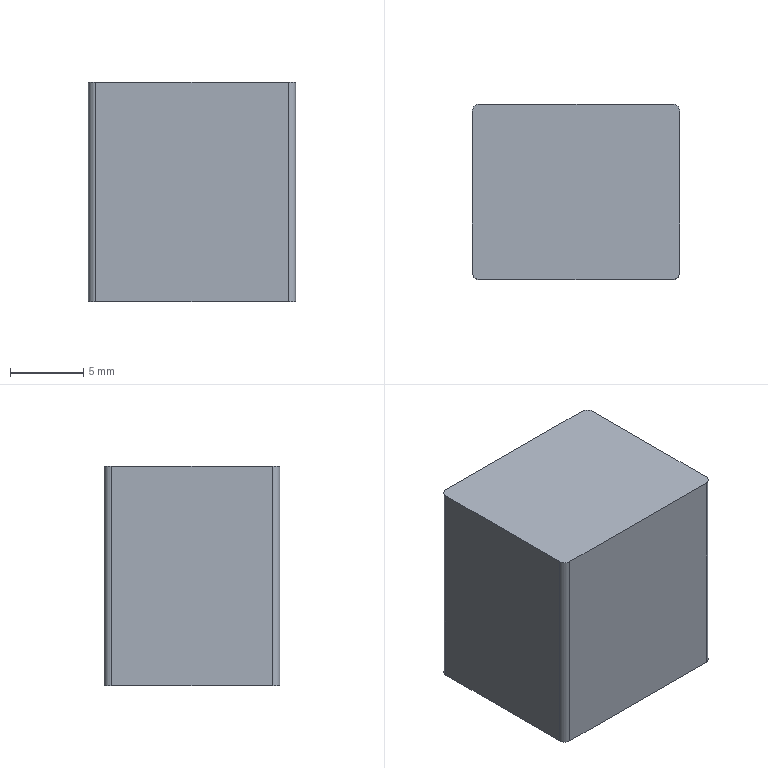Part | NX | features BREP 1 | 1 solid | 10 faces | box 14.163 x 11.999 x 15 mm | volume 2546 mm3 | plane 6 | cylinder 4 | commonest cylinder face diameters 1 x4
STEP:
#1=CARTESIAN_POINT('',(-6.581,6.,-25.6));
#2=VERTEX_POINT('',#1);
#3=CARTESIAN_POINT('',(-7.081,5.5,-25.6));
#4=VERTEX_POINT('',#3);
#5=CARTESIAN_POINT('',(-6.581,5.5,-25.6));
#6=DIRECTION('',(0.,0.,1.));
#7=DIRECTION('',(1.,0.,0.));
#8=AXIS2_PLACEMENT_3D('',#5,#6,#7);
#9=CIRCLE('',#8,0.5);
#10=EDGE_CURVE('',#2,#4,#9,.T.);
#11=ORIENTED_EDGE('',*,*,#10,.F.);
#12=CARTESIAN_POINT('',(-6.581,6.,-40.6));
#13=VERTEX_POINT('',#12);
#14=CARTESIAN_POINT('',(-6.581,6.,-40.6));
#15=DIRECTION('',(0.,0.,1.));
#16=VECTOR('',#15,1000.);
#17=LINE('',#14,#16);
#18=EDGE_CURVE('',#13,#2,#17,.T.);
#19=ORIENTED_EDGE('',*,*,#18,.F.);
#20=CARTESIAN_POINT('',(-7.081,5.5,-40.6));
#21=VERTEX_POINT('',#20);
#22=CARTESIAN_POINT('',(-6.581,5.5,-40.6));
#23=DIRECTION('',(0.,0.,1.));
#24=DIRECTION('',(1.,0.,0.));
#25=AXIS2_PLACEMENT_3D('',#22,#23,#24);
#26=CIRCLE('',#25,0.5);
#27=EDGE_CURVE('',#13,#21,#26,.T.);
#28=ORIENTED_EDGE('',*,*,#27,.T.);
#29=CARTESIAN_POINT('',(-7.081,5.5,-40.6));
#30=DIRECTION('',(0.,0.,1.));
#31=VECTOR('',#30,1000.);
#32=LINE('',#29,#31);
#33=EDGE_CURVE('',#21,#4,#32,.T.);
#34=ORIENTED_EDGE('',*,*,#33,.T.);
#35=EDGE_LOOP('',(#11,#19,#28,#34));
#36=FACE_BOUND('',#35,.T.);
#37=CARTESIAN_POINT('',(-6.581,5.5,-40.6));
#38=DIRECTION('',(0.,0.,1.));
#39=DIRECTION('',(-1.,0.,0.));
#40=AXIS2_PLACEMENT_3D('',#37,#38,#39);
#41=CYLINDRICAL_SURFACE('',#40,0.5);
#42=ADVANCED_FACE('',(#36),#41,.T.);
#43=CARTESIAN_POINT('',(-7.081,-5.5,-25.6));
#44=VERTEX_POINT('',#43);
#45=CARTESIAN_POINT('',(-7.081,-5.5,-25.6));
#46=DIRECTION('',(0.,1.,0.));
#47=VECTOR('',#46,1000.);
#48=LINE('',#45,#47);
#49=EDGE_CURVE('',#44,#4,#48,.T.);
#50=ORIENTED_EDGE('',*,*,#49,.T.);
#51=ORIENTED_EDGE('',*,*,#33,.F.);
#52=CARTESIAN_POINT('',(-7.081,-5.5,-40.6));
#53=VERTEX_POINT('',#52);
#54=CARTESIAN_POINT('',(-7.081,-5.5,-40.6));
#55=DIRECTION('',(0.,1.,0.));
#56=VECTOR('',#55,1000.);
#57=LINE('',#54,#56);
#58=EDGE_CURVE('',#53,#21,#57,.T.);
#59=ORIENTED_EDGE('',*,*,#58,.F.);
#60=CARTESIAN_POINT('',(-7.081,-5.5,-40.6));
#61=DIRECTION('',(0.,0.,1.));
#62=VECTOR('',#61,1000.);
#63=LINE('',#60,#62);
#64=EDGE_CURVE('',#53,#44,#63,.T.);
#65=ORIENTED_EDGE('',*,*,#64,.T.);
#66=EDGE_LOOP('',(#50,#51,#59,#65));
#67=FACE_BOUND('',#66,.T.);
#68=CARTESIAN_POINT('',(-7.081,-5.5,-40.6));
#69=DIRECTION('',(1.,0.,0.));
#70=DIRECTION('',(0.,0.,1.));
#71=AXIS2_PLACEMENT_3D('',#68,#69,#70);
#72=PLANE('',#71);
#73=ADVANCED_FACE('',(#67),#72,.F.);
#74=CARTESIAN_POINT('',(-6.581,-6.,-25.6));
#75=VERTEX_POINT('',#74);
#76=CARTESIAN_POINT('',(-6.581,-5.5,-25.6));
#77=DIRECTION('',(0.,0.,1.));
#78=DIRECTION('',(1.,0.,0.));
#79=AXIS2_PLACEMENT_3D('',#76,#77,#78);
#80=CIRCLE('',#79,0.5);
#81=EDGE_CURVE('',#44,#75,#80,.T.);
#82=ORIENTED_EDGE('',*,*,#81,.F.);
#83=ORIENTED_EDGE('',*,*,#64,.F.);
#84=CARTESIAN_POINT('',(-6.581,-6.,-40.6));
#85=VERTEX_POINT('',#84);
#86=CARTESIAN_POINT('',(-6.581,-5.5,-40.6));
#87=DIRECTION('',(0.,0.,1.));
#88=DIRECTION('',(1.,0.,0.));
#89=AXIS2_PLACEMENT_3D('',#86,#87,#88);
#90=CIRCLE('',#89,0.5);
#91=EDGE_CURVE('',#53,#85,#90,.T.);
#92=ORIENTED_EDGE('',*,*,#91,.T.);
#93=CARTESIAN_POINT('',(-6.581,-6.,-40.6));
#94=DIRECTION('',(0.,0.,1.));
#95=VECTOR('',#94,1000.);
#96=LINE('',#93,#95);
#97=EDGE_CURVE('',#85,#75,#96,.T.);
#98=ORIENTED_EDGE('',*,*,#97,.T.);
#99=EDGE_LOOP('',(#82,#83,#92,#98));
#100=FACE_BOUND('',#99,.T.);
#101=CARTESIAN_POINT('',(-6.581,-5.5,-40.6));
#102=DIRECTION('',(0.,0.,1.));
#103=DIRECTION('',(-1.,0.,0.));
#104=AXIS2_PLACEMENT_3D('',#101,#102,#103);
#105=CYLINDRICAL_SURFACE('',#104,0.5);
#106=ADVANCED_FACE('',(#100),#105,.T.);
#107=CARTESIAN_POINT('',(6.581,-6.,-25.6));
#108=VERTEX_POINT('',#107);
#109=CARTESIAN_POINT('',(6.581,-6.,-25.6));
#110=DIRECTION('',(-1.,0.,0.));
#111=VECTOR('',#110,1000.);
#112=LINE('',#109,#111);
#113=EDGE_CURVE('',#108,#75,#112,.T.);
#114=ORIENTED_EDGE('',*,*,#113,.T.);
#115=ORIENTED_EDGE('',*,*,#97,.F.);
#116=CARTESIAN_POINT('',(6.581,-6.,-40.6));
#117=VERTEX_POINT('',#116);
#118=CARTESIAN_POINT('',(6.581,-6.,-40.6));
#119=DIRECTION('',(-1.,0.,0.));
#120=VECTOR('',#119,1000.);
#121=LINE('',#118,#120);
#122=EDGE_CURVE('',#117,#85,#121,.T.);
#123=ORIENTED_EDGE('',*,*,#122,.F.);
#124=CARTESIAN_POINT('',(6.581,-6.,-40.6));
#125=DIRECTION('',(0.,0.,1.));
#126=VECTOR('',#125,1000.);
#127=LINE('',#124,#126);
#128=EDGE_CURVE('',#117,#108,#127,.T.);
#129=ORIENTED_EDGE('',*,*,#128,.T.);
#130=EDGE_LOOP('',(#114,#115,#123,#129));
#131=FACE_BOUND('',#130,.T.);
#132=CARTESIAN_POINT('',(6.581,-6.,-40.6));
#133=DIRECTION('',(0.,1.,0.));
#134=DIRECTION('',(0.,0.,-1.));
#135=AXIS2_PLACEMENT_3D('',#132,#133,#134);
#136=PLANE('',#135);
#137=ADVANCED_FACE('',(#131),#136,.F.);
#138=CARTESIAN_POINT('',(7.081,-5.5,-25.6));
#139=VERTEX_POINT('',#138);
#140=CARTESIAN_POINT('',(6.581,-5.5,-25.6));
#141=DIRECTION('',(0.,0.,1.));
#142=DIRECTION('',(1.,0.,0.));
#143=AXIS2_PLACEMENT_3D('',#140,#141,#142);
#144=CIRCLE('',#143,0.5);
#145=EDGE_CURVE('',#108,#139,#144,.T.);
#146=ORIENTED_EDGE('',*,*,#145,.F.);
#147=ORIENTED_EDGE('',*,*,#128,.F.);
#148=CARTESIAN_POINT('',(7.081,-5.5,-40.6));
#149=VERTEX_POINT('',#148);
#150=CARTESIAN_POINT('',(6.581,-5.5,-40.6));
#151=DIRECTION('',(0.,0.,1.));
#152=DIRECTION('',(1.,0.,0.));
#153=AXIS2_PLACEMENT_3D('',#150,#151,#152);
#154=CIRCLE('',#153,0.5);
#155=EDGE_CURVE('',#117,#149,#154,.T.);
#156=ORIENTED_EDGE('',*,*,#155,.T.);
#157=CARTESIAN_POINT('',(7.081,-5.5,-40.6));
#158=DIRECTION('',(0.,0.,1.));
#159=VECTOR('',#158,1000.);
#160=LINE('',#157,#159);
#161=EDGE_CURVE('',#149,#139,#160,.T.);
#162=ORIENTED_EDGE('',*,*,#161,.T.);
#163=EDGE_LOOP('',(#146,#147,#156,#162));
#164=FACE_BOUND('',#163,.T.);
#165=CARTESIAN_POINT('',(6.581,-5.5,-40.6));
#166=DIRECTION('',(0.,0.,1.));
#167=DIRECTION('',(-1.,0.,0.));
#168=AXIS2_PLACEMENT_3D('',#165,#166,#167);
#169=CYLINDRICAL_SURFACE('',#168,0.5);
#170=ADVANCED_FACE('',(#164),#169,.T.);
#171=CARTESIAN_POINT('',(7.081,5.5,-25.6));
#172=VERTEX_POINT('',#171);
#173=CARTESIAN_POINT('',(7.081,5.5,-25.6));
#174=DIRECTION('',(0.,-1.,0.));
#175=VECTOR('',#174,1000.);
#176=LINE('',#173,#175);
#177=EDGE_CURVE('',#172,#139,#176,.T.);
#178=ORIENTED_EDGE('',*,*,#177,.T.);
#179=ORIENTED_EDGE('',*,*,#161,.F.);
#180=CARTESIAN_POINT('',(7.081,5.5,-40.6));
#181=VERTEX_POINT('',#180);
#182=CARTESIAN_POINT('',(7.081,5.5,-40.6));
#183=DIRECTION('',(0.,-1.,0.));
#184=VECTOR('',#183,1000.);
#185=LINE('',#182,#184);
#186=EDGE_CURVE('',#181,#149,#185,.T.);
#187=ORIENTED_EDGE('',*,*,#186,.F.);
#188=CARTESIAN_POINT('',(7.081,5.5,-40.6));
#189=DIRECTION('',(0.,0.,1.));
#190=VECTOR('',#189,1000.);
#191=LINE('',#188,#190);
#192=EDGE_CURVE('',#181,#172,#191,.T.);
#193=ORIENTED_EDGE('',*,*,#192,.T.);
#194=EDGE_LOOP('',(#178,#179,#187,#193));
#195=FACE_BOUND('',#194,.T.);
#196=CARTESIAN_POINT('',(7.081,5.5,-40.6));
#197=DIRECTION('',(-1.,0.,0.));
#198=DIRECTION('',(0.,0.,-1.));
#199=AXIS2_PLACEMENT_3D('',#196,#197,#198);
#200=PLANE('',#199);
#201=ADVANCED_FACE('',(#195),#200,.F.);
#202=CARTESIAN_POINT('',(6.581,6.,-25.6));
#203=VERTEX_POINT('',#202);
#204=CARTESIAN_POINT('',(6.581,5.5,-25.6));
#205=DIRECTION('',(0.,0.,1.));
#206=DIRECTION('',(1.,0.,0.));
#207=AXIS2_PLACEMENT_3D('',#204,#205,#206);
#208=CIRCLE('',#207,0.5);
#209=EDGE_CURVE('',#172,#203,#208,.T.);
#210=ORIENTED_EDGE('',*,*,#209,.F.);
#211=ORIENTED_EDGE('',*,*,#192,.F.);
#212=CARTESIAN_POINT('',(6.581,6.,-40.6));
#213=VERTEX_POINT('',#212);
#214=CARTESIAN_POINT('',(6.581,5.5,-40.6));
#215=DIRECTION('',(0.,0.,1.));
#216=DIRECTION('',(1.,0.,0.));
#217=AXIS2_PLACEMENT_3D('',#214,#215,#216);
#218=CIRCLE('',#217,0.5);
#219=EDGE_CURVE('',#181,#213,#218,.T.);
#220=ORIENTED_EDGE('',*,*,#219,.T.);
#221=CARTESIAN_POINT('',(6.581,6.,-40.6));
#222=DIRECTION('',(0.,0.,1.));
#223=VECTOR('',#222,1000.);
#224=LINE('',#221,#223);
#225=EDGE_CURVE('',#213,#203,#224,.T.);
#226=ORIENTED_EDGE('',*,*,#225,.T.);
#227=EDGE_LOOP('',(#210,#211,#220,#226));
#228=FACE_BOUND('',#227,.T.);
#229=CARTESIAN_POINT('',(6.581,5.5,-40.6));
#230=DIRECTION('',(0.,0.,1.));
#231=DIRECTION('',(-1.,0.,0.));
#232=AXIS2_PLACEMENT_3D('',#229,#230,#231);
#233=CYLINDRICAL_SURFACE('',#232,0.5);
#234=ADVANCED_FACE('',(#228),#233,.T.);
#235=CARTESIAN_POINT('',(-6.581,6.,-25.6));
#236=DIRECTION('',(1.,0.,0.));
#237=VECTOR('',#236,1000.);
#238=LINE('',#235,#237);
#239=EDGE_CURVE('',#2,#203,#238,.T.);
#240=ORIENTED_EDGE('',*,*,#239,.T.);
#241=ORIENTED_EDGE('',*,*,#225,.F.);
#242=CARTESIAN_POINT('',(-6.581,6.,-40.6));
#243=DIRECTION('',(1.,0.,0.));
#244=VECTOR('',#243,1000.);
#245=LINE('',#242,#244);
#246=EDGE_CURVE('',#13,#213,#245,.T.);
#247=ORIENTED_EDGE('',*,*,#246,.F.);
#248=ORIENTED_EDGE('',*,*,#18,.T.);
#249=EDGE_LOOP('',(#240,#241,#247,#248));
#250=FACE_BOUND('',#249,.T.);
#251=CARTESIAN_POINT('',(-6.581,6.,-40.6));
#252=DIRECTION('',(0.,-1.,0.));
#253=DIRECTION('',(0.,0.,1.));
#254=AXIS2_PLACEMENT_3D('',#251,#252,#253);
#255=PLANE('',#254);
#256=ADVANCED_FACE('',(#250),#255,.F.);
#257=ORIENTED_EDGE('',*,*,#27,.F.);
#258=ORIENTED_EDGE('',*,*,#246,.T.);
#259=ORIENTED_EDGE('',*,*,#219,.F.);
#260=ORIENTED_EDGE('',*,*,#186,.T.);
#261=ORIENTED_EDGE('',*,*,#155,.F.);
#262=ORIENTED_EDGE('',*,*,#122,.T.);
#263=ORIENTED_EDGE('',*,*,#91,.F.);
#264=ORIENTED_EDGE('',*,*,#58,.T.);
#265=EDGE_LOOP('',(#257,#258,#259,#260,#261,#262,#263,#264));
#266=FACE_BOUND('',#265,.T.);
#267=CARTESIAN_POINT('',(-6.581,5.5,-40.6));
#268=DIRECTION('',(0.,0.,1.));
#269=DIRECTION('',(-1.,0.,0.));
#270=AXIS2_PLACEMENT_3D('',#267,#268,#269);
#271=PLANE('',#270);
#272=ADVANCED_FACE('',(#266),#271,.F.);
#273=ORIENTED_EDGE('',*,*,#10,.T.);
#274=ORIENTED_EDGE('',*,*,#49,.F.);
#275=ORIENTED_EDGE('',*,*,#81,.T.);
#276=ORIENTED_EDGE('',*,*,#113,.F.);
#277=ORIENTED_EDGE('',*,*,#145,.T.);
#278=ORIENTED_EDGE('',*,*,#177,.F.);
#279=ORIENTED_EDGE('',*,*,#209,.T.);
#280=ORIENTED_EDGE('',*,*,#239,.F.);
#281=EDGE_LOOP('',(#273,#274,#275,#276,#277,#278,#279,#280));
#282=FACE_BOUND('',#281,.T.);
#283=CARTESIAN_POINT('',(-6.581,5.5,-25.6));
#284=DIRECTION('',(0.,0.,1.));
#285=DIRECTION('',(-1.,0.,0.));
#286=AXIS2_PLACEMENT_3D('',#283,#284,#285);
#287=PLANE('',#286);
#288=ADVANCED_FACE('',(#282),#287,.T.);
#289=CLOSED_SHELL('',(#42,#73,#106,#137,#170,#201,#234,#256,#272,#288));
#290=MANIFOLD_SOLID_BREP('',#289);
#291=(LENGTH_UNIT()NAMED_UNIT(*)SI_UNIT(.MILLI.,.METRE.));
#292=UNCERTAINTY_MEASURE_WITH_UNIT(LENGTH_MEASURE(0.00001),#291,'','');
#293=(NAMED_UNIT(*)PLANE_ANGLE_UNIT()SI_UNIT($,.RADIAN.));
#294=(NAMED_UNIT(*)SI_UNIT($,.STERADIAN.)SOLID_ANGLE_UNIT());
#295=(GEOMETRIC_REPRESENTATION_CONTEXT(3)GLOBAL_UNCERTAINTY_ASSIGNED_CONTEXT((#292))GLOBAL_UNIT_ASSIGNED_CONTEXT((#291,#293,#294))REPRESENTATION_CONTEXT('',''));
#296=ADVANCED_BREP_SHAPE_REPRESENTATION('',(#290),#295);